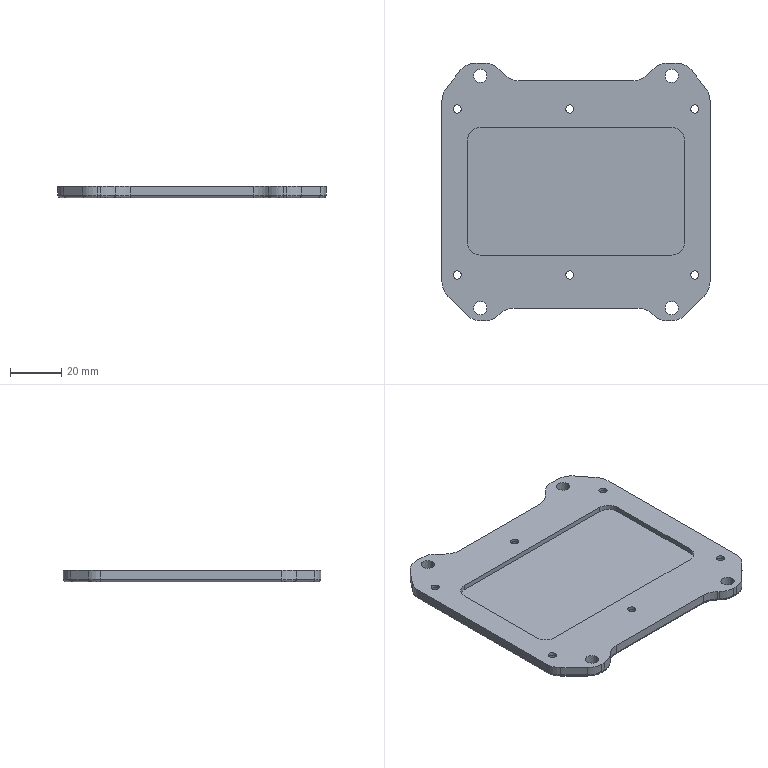NC program | NX | posted with a generic post | part box 105 x 101 x 4.5 mm
Lines 3985 to 4891 of 30641:
(CURVE_DRIVE , TOOL : 球刀R1-4-D4-50)
N7932 T08 M6
N7934 G53
N7936 G17 G0 G90 X36.658 Y51.5 S4500 M3
N7938 G43 Z20. H8
N7940 Z2.579
N7942 G94 G1 Z-1. F2500.
N7944 X36.668 Z-1.142
N7946 X36.698 Z-1.282
N7948 X36.748 Z-1.415
N7950 X36.817 Z-1.541
N7952 X36.902 Z-1.655
N7954 X37.003 Z-1.756
N7956 X37.117 Z-1.841
N7958 X37.242 Z-1.91
N7960 X37.376 Z-1.959
N7962 X37.516 Z-1.99
N7964 X37.658 Z-2.
N7966 X39.193
N7968 X39.348 Y51.498
N7970 X39.503 Y51.494
N7972 X39.658 Y51.488
N7974 X39.968 Y51.466
N7976 X40.157 Y51.447
N7978 X40.433 Y51.413
N7980 G2 X46.277 Y48.043 R9.005
N7982 G1 X51.587 Y41.282
N7984 G2 X53.5 Y35.665 R9.008
N7986 G1 Y-35.201
N7988 G2 X51.02 Y-41.39 R9.002
N7990 G1 X50.864 Y-41.55 Z-2.001
N7992 X50.843 Y-41.571 Z-2.007
N7994 X50.825 Y-41.589 Z-2.003
N7996 X43.531 Y-48.883 Z-2.
N7998 G2 X40.952 Y-50.674 R9.036
N8000 G1 X40.897 Y-50.699 Z-2.001
N8002 X40.833 Y-50.727 Z-2.002
N8004 X40.688 Y-50.79 Z-2.001
N8006 X40.588 Y-50.832 Z-2.
N8008 X40.433 Y-50.894
N8010 G2 X37.18 Y-51.5 R9.002
N8012 G1 X35.785
N8014 G2 X29.434 Y-48.848 R9.004
N8016 G1 X29.124 Y-48.539
N8018 G3 X24.39 Y-46.504 R6.999
N8020 G1 X24.322 Y-46.502 Z-2.001
N8022 X24.167 Y-46.5 Z-2.004
N8024 X24.08 Z-2.006
N8026 X23.925 Z-2.002
N8028 X-24.167 Z-2.
N8030 G3 X-29.124 Y-48.539 R7.002
N8032 G1 X-29.434 Y-48.848
N8034 G2 X-31.912 Y-50.61 R9.023
N8036 G1 X-32.048 Y-50.674 Z-2.001
N8038 X-32.167 Y-50.727 Z-2.002
N8040 X-32.222 Y-50.752 Z-2.001
N8042 X-32.377 Y-50.818 Z-2.
N8044 X-32.532 Y-50.88
N8046 G2 X-35.785 Y-51.5 R9.056
N8048 G1 X-37.18
N8050 G2 X-43.531 Y-48.883 R9.005
N8052 G1 X-50.87 Y-41.545
N8054 G2 X-53.5 Y-35.201 R9.006
N8056 G1 Y35.665
N8058 G2 X-51.502 Y41.39 R9.017
N8060 G1 X-46.277 Y48.043
N8062 G2 X-40.433 Y51.413 R9.005
N8064 G1 X-40.158 Y51.447
N8066 X-39.968 Y51.466
N8068 X-39.658 Y51.488
N8070 X-39.503 Y51.494
N8072 X-39.348 Y51.498
N8074 X-39.193 Y51.5
N8076 X-35.785
N8078 G2 X-29.434 Y48.848 R9.004
N8080 G1 X-27.236 Y46.651
N8082 G3 X-25.641 Y45.413 R7.073
N8084 G1 X-25.561 Y45.368
N8086 G3 X-22.153 Y44.5 R6.993
N8088 G1 X22.153
N8090 G3 X27.11 Y46.525 R6.998
N8092 G1 X27.786 Y47.2
N8094 X29.434 Y48.848
N8096 G2 X31.912 Y50.61 R9.023
N8098 G1 X32.048 Y50.674 Z-2.001
N8100 X32.167 Y50.727 Z-2.002
N8102 X32.222 Y50.752 Z-2.001
N8104 X32.287 Y50.78 Z-2.
N8106 G2 X35.785 Y51.5 R8.987
N8108 G1 X37.658
N8110 Y51.499 Z-1.969
N8112 Y51.497 Z-1.92
N8114 X39.193
N8116 X39.348 Y51.495
N8118 X39.503 Y51.491
N8120 X39.658 Y51.485
N8122 X39.968 Y51.463
N8124 X40.154 Y51.445
N8126 X40.356 Y51.42
N8128 G2 X42.137 Y51. R9.113
N8130 G1 X42.187 Y50.983
N8132 G2 X43.267 Y50.519 R9.54
N8134 G1 X43.376 Y50.462
N8136 X43.55 Y50.368
N8138 X43.558 Y50.364
N8140 G2 X44.303 Y49.9 R8.898
N8142 G1 X44.461 Y49.789
N8144 G2 X46.303 Y48.006 R9.094
N8146 G1 X46.638 Y47.579
N8148 G3 X48.825 Y44.794 R3917.638
N8150 G1 X48.947 Y44.639
N8152 X48.953 Y44.631
N8154 X49.56 Y43.859
N8156 X49.676 Y43.711
N8158 G2 X50.988 Y42.04 R9051.305
N8160 G1 X51.255 Y41.699
N8162 G2 X51.742 Y41.074 R21.302
N8164 G1 X51.794 Y40.999
N8166 G2 X52.655 Y39.533 R8.658
N8168 G1 X52.667 Y39.511
N8170 G2 X53.291 Y37.654 R9.165
N8172 G1 X53.3 Y37.601
N8174 G2 X53.493 Y35.974 R8.95
N8176 G1 X53.495 Y35.896
N8178 X53.497 Y35.82
N8180 X53.496 Y35.746
N8182 X53.497 Y35.665
N8184 Y-35.201
N8186 G2 X53.462 Y-35.974 R8.462
N8188 G1 X53.445 Y-36.159
N8190 G2 X53.051 Y-37.986 R8.987
N8192 G1 X52.989 Y-38.166
N8194 X52.981 Y-38.192
N8196 G2 X51.288 Y-41.092 R9.015
N8198 G1 X51.161 Y-41.235
N8200 X51.017 Y-41.39
N8202 X50.866 Y-41.545 Z-1.921
N8204 X50.836 Y-41.575 Z-1.925
N8206 X50.812 Y-41.599 Z-1.923
N8208 X43.593 Y-48.817 Z-1.92
N8210 G2 X41.003 Y-50.646 R9.001
N8212 G1 X40.932 Y-50.681
N8214 X40.814 Y-50.733 Z-1.922
N8216 X40.715 Y-50.776 Z-1.921
N8218 X40.687 Y-50.787
N8220 X40.592 Y-50.829 Z-1.92
N8222 X40.588 Y-50.83
N8224 X40.433 Y-50.891
N8226 G2 X38.884 Y-51.336 R8.857
N8228 G1 X38.794 Y-51.352
N8230 G2 X37.18 Y-51.497 R8.944
N8232 G1 X35.785
N8234 G2 X33.839 Y-51.278 R8.977
N8236 G1 X33.678 Y-51.239
N8238 G2 X31.448 Y-50.366 R8.951
N8240 G1 X31.442 Y-50.364
N8242 X31.381 Y-50.328
N8244 G2 X30.318 Y-49.624 R8.845
N8246 G1 X30.249 Y-49.57
N8248 G2 X29.872 Y-49.256 R8.905
N8250 G1 X29.826 Y-49.214
N8252 X29.744 Y-49.14
N8254 X29.735 Y-49.133
N8256 X29.578 Y-48.985
N8258 X29.406 Y-48.817
N8260 X29.124 Y-48.535
N8262 G3 X25.096 Y-46.557 R7.005
N8264 G1 X24.941 Y-46.538
N8266 X24.786 Y-46.524
N8268 X24.631 Y-46.512
N8270 X24.477 Y-46.504
N8272 X24.393 Y-46.501
N8274 X24.322 Y-46.499 Z-1.921
N8276 X24.243 Z-1.922
N8278 X24.167 Y-46.498 Z-1.924
N8280 X24.085 Z-1.926
N8282 X23.925 Z-1.922
N8284 X-24.167 Z-1.92
N8286 G3 X-26.955 Y-47.068 R7.018
N8288 G1 X-27.077 Y-47.123
N8290 X-27.11 Y-47.137
N8292 G3 X-29.124 Y-48.535 R7.012
N8294 G1 X-29.434 Y-48.844
N8296 G2 X-30.082 Y-49.436 R10.496
N8298 G1 X-30.147 Y-49.487
N8300 G2 X-30.495 Y-49.756 R6.75
N8302 G1 X-30.518 Y-49.773
N8304 G2 X-31.381 Y-50.328 R8.373
N8306 G1 X-31.445 Y-50.365
N8308 X-31.448 Y-50.366
N8310 X-31.603 Y-50.451
N8312 X-31.733 Y-50.519
N8314 X-31.741 Y-50.522
N8316 X-31.912 Y-50.607
N8318 X-32.062 Y-50.678 Z-1.921
N8320 X-32.067 Y-50.679
N8322 X-32.146 Y-50.715 Z-1.922
N8324 X-32.222 Y-50.749
N8326 X-32.276 Y-50.771 Z-1.921
N8328 X-32.377 Y-50.815
N8330 X-32.409 Y-50.828 Z-1.92
N8332 X-32.532 Y-50.877
N8334 G2 X-34.856 Y-51.446 R8.986
N8336 G1 X-34.863 Y-51.447
N8338 G2 X-35.785 Y-51.497 R9.145
N8340 G1 X-37.18
N8342 G2 X-40.588 Y-50.83 R8.992
N8344 G1 X-40.595 Y-50.827
N8346 G2 X-41.052 Y-50.624 R13.008
N8348 G1 X-41.245 Y-50.529
N8350 X-41.267 Y-50.519
N8352 G2 X-42.295 Y-49.906 R9.146
N8354 G1 X-42.495 Y-49.765
N8356 G2 X-43.531 Y-48.879 R9.388
N8358 G1 X-46.378 Y-46.032
N8360 X-50.866 Y-41.545
N8362 G2 X-53.229 Y-37.367 R9.014
N8364 G1 X-53.245 Y-37.296
N8366 G2 X-53.474 Y-35.82 R8.914
N8368 G1 X-53.484 Y-35.665
N8370 X-53.49 Y-35.51
N8372 X-53.495 Y-35.356
N8374 X-53.497 Y-35.201
N8376 Y35.665
N8378 G2 X-53.445 Y36.706 R9.699
N8380 G1 X-53.433 Y36.802
N8382 G2 X-53.196 Y38.039 R8.303
N8384 G1 X-53.17 Y38.141
N8386 G2 X-52.856 Y39.069 R9.602
N8388 G1 X-52.82 Y39.159
N8390 G2 X-51.896 Y40.857 R9.054
N8392 G1 X-51.848 Y40.926
N8394 G2 X-51.267 Y41.684 R16.261
N8396 G1 X-51.126 Y41.864
N8398 G2 X-49.708 Y43.67 R1437.629
N8400 G1 X-49.573 Y43.842
N8402 G3 X-47.249 Y46.802 R3035.735
N8404 G1 X-47.124 Y46.96
N8406 X-47.094 Y46.999
N8408 X-46.759 Y47.424
N8410 X-46.635 Y47.583
N8412 X-46.303 Y48.006
N8414 G2 X-45.39 Y49.016 R9.198
N8416 G1 X-45.332 Y49.07
N8418 G2 X-43.686 Y50.291 R8.897
N8420 G1 X-43.558 Y50.364
N8422 X-43.55 Y50.368
N8424 G2 X-42.941 Y50.677 R8.914
N8426 G1 X-42.86 Y50.712
N8428 G2 X-41.982 Y51.052 R9.144
N8430 G1 X-41.914 Y51.072
N8432 X-41.706 Y51.138
N8434 G2 X-40.278 Y51.43 R9.209
N8436 G1 X-40.138 Y51.447
N8438 X-39.968 Y51.463
N8440 X-39.658 Y51.485
N8442 X-39.503 Y51.491
N8444 X-39.348 Y51.495
N8446 X-39.193 Y51.497
N8448 X-35.785
N8450 G2 X-33.839 Y51.278 R8.977
N8452 G1 X-33.678 Y51.239
N8454 G2 X-31.448 Y50.366 R8.951
N8456 G1 X-31.442 Y50.364
N8458 X-31.381 Y50.328
N8460 G2 X-30.318 Y49.624 R8.845
N8462 G1 X-30.249 Y49.57
N8464 G2 X-29.872 Y49.256 R8.905
N8466 G1 X-29.826 Y49.214
N8468 X-29.744 Y49.14
N8470 X-29.735 Y49.133
N8472 X-29.578 Y48.985
N8474 X-29.406 Y48.817
N8476 X-27.24 Y46.651
N8478 G3 X-25.871 Y45.546 R7.094
N8480 G1 X-25.8 Y45.504
N8482 G3 X-23.492 Y44.621 R6.981
N8484 G1 X-23.392 Y44.602
N8486 G3 X-22.153 Y44.498 R7.183
N8488 G1 X22.153
N8490 G3 X24.199 Y44.794 R6.901
N8492 G1 X24.322 Y44.831
N8494 G3 X27.099 Y46.51 R7.007
N8496 G1 X27.33 Y46.741
N8498 X29.434 Y48.844
N8500 G2 X30.082 Y49.436 R10.496
N8502 G1 X30.147 Y49.487
N8504 G2 X30.495 Y49.756 R6.751
N8506 G1 X30.518 Y49.773
N8508 G2 X31.381 Y50.328 R8.374
N8510 G1 X31.445 Y50.365
N8512 X31.448 Y50.366
N8514 X31.603 Y50.451
N8516 X31.733 Y50.519
N8518 X31.741 Y50.522
N8520 X31.912 Y50.607
N8522 X32.062 Y50.678 Z-1.921
N8524 X32.067 Y50.679
N8526 X32.146 Y50.715 Z-1.922
N8528 X32.222 Y50.749 Z-1.921
N8530 X32.277 Y50.772 Z-1.92
N8532 X32.377 Y50.815
N8534 X32.409 Y50.828
N8536 X32.532 Y50.877
N8538 G2 X34.856 Y51.446 R8.986
N8540 G1 X34.863 Y51.447
N8542 G2 X35.785 Y51.497 R9.145
N8544 G1 X37.658
N8546 Y51.493 Z-1.84
N8548 X39.191
N8550 X39.348 Y51.491
N8552 X39.537 Y51.486
N8554 X39.658 Y51.481
N8556 X39.871 Y51.466
N8558 X39.968 Y51.459
N8560 X40.087 Y51.447
N8562 X40.278 Y51.426
N8564 X40.433 Y51.406
N8566 G2 X42.791 Y50.737 R8.941
N8568 G1 X42.925 Y50.679
N8570 G2 X46.292 Y48.013 R9.018
N8572 G1 X47.483 Y46.496
N8574 X49.966 Y43.334
N8576 X50.037 Y43.243
N8578 X50.396 Y42.787
N8580 X51.587 Y41.271
N8582 G2 X53.129 Y38.265 R8.995
N8584 G1 X53.153 Y38.183
N8586 G2 X53.493 Y35.665 R8.998
N8588 G1 Y-35.201
N8590 G2 X51.011 Y-41.39 R9.
N8592 G1 X50.86 Y-41.545 Z-1.841
N8594 X50.849 Y-41.556 Z-1.843
N8596 X50.784 Y-41.621
N8598 X43.519 Y-48.886 Z-1.84
N8600 G2 X41.052 Y-50.62 R9.021
N8602 G1 X40.898 Y-50.691 Z-1.841
N8604 X40.743 Y-50.76
N8606 X40.656 Y-50.796
N8608 X40.619 Y-50.811
N8610 X40.578 Y-50.828 Z-1.84
N8612 X40.433 Y-50.887
N8614 G2 X37.182 Y-51.493 R9.021
N8616 G1 X35.788
N8618 G2 X29.415 Y-48.82 R9.001
N8620 G1 X29.104 Y-48.51
N8622 G3 X24.477 Y-46.5 R7.006
N8624 G1 X24.322 Y-46.495 Z-1.841
N8626 X24.167 Y-46.493 Z-1.844
N8628 X24.124 Z-1.845
N8630 X24.012 Z-1.844
N8632 X23.966 Z-1.843
N8634 X23.857 Z-1.842
N8636 X-24.167 Z-1.84
N8638 G3 X-29.124 Y-48.529 R7.014
N8640 G1 X-29.434 Y-48.839
N8642 G2 X-31.912 Y-50.602 R8.989
N8644 G1 X-32.064 Y-50.674 Z-1.841
N8646 X-32.067 Y-50.675
N8648 X-32.139 Y-50.707 Z-1.842
N8650 X-32.222 Y-50.745
N8652 X-32.298 Y-50.777 Z-1.841
N8654 X-32.377 Y-50.81
N8656 X-32.41 Y-50.824 Z-1.84
N8658 X-32.532 Y-50.873
N8660 G2 X-35.785 Y-51.493 R9.042
N8662 G1 X-37.18
N8664 G2 X-43.531 Y-48.874 R9.002
N8666 G1 X-50.86 Y-41.545
N8668 G2 X-53.493 Y-35.201 R8.997
N8670 G1 Y35.683
N8672 G2 X-51.587 Y41.271 R9.003
N8674 G1 X-50.159 Y43.089
N8676 X-50.035 Y43.247
N8678 X-49.227 Y44.276
N8680 X-47.404 Y46.597
N8682 X-46.268 Y48.043
N8684 G2 X-42.925 Y50.679 R9.013
N8686 G1 X-42.791 Y50.737
N8688 X-42.756 Y50.753
N8690 G2 X-40.278 Y51.426 R8.982
N8692 G1 X-40.068 Y51.449
N8694 X-39.968 Y51.459
N8696 X-39.752 Y51.475
N8698 X-39.658 Y51.481
N8700 X-39.481 Y51.488
N8702 X-39.348 Y51.491
N8704 X-39.193 Y51.493
N8706 X-35.788
N8708 G2 X-29.415 Y48.82 R9.001
N8710 G1 X-27.153 Y46.559
N8712 G3 X-22.153 Y44.493 R7.009
N8714 G1 X22.153
N8716 G3 X27.11 Y46.516 R7.013
N8718 G1 X27.415 Y46.82
N8720 X29.434 Y48.839
N8722 G2 X31.912 Y50.602 R8.989
N8724 G1 X32.064 Y50.674 Z-1.841
N8726 X32.067 Y50.675
N8728 X32.139 Y50.707 Z-1.842
N8730 X32.222 Y50.745 Z-1.841
N8732 X32.301 Y50.778 Z-1.84
N8734 G2 X35.785 Y51.493 R8.987
N8736 G1 X37.658
N8738 Y51.486 Z-1.766
N8740 Y51.485 Z-1.761
N8742 X39.193
N8744 X39.348 Y51.483
N8746 X39.503 Y51.479
N8748 X39.658 Y51.472
N8750 X39.712 Y51.468
N8752 X39.821 Y51.462 Z-1.76
N8754 G2 X40.445 Y51.396 R9.361
N8756 G1 X40.588 Y51.374 Z-1.761
N8758 G2 X46.137 Y48.193 R8.982
N8760 G1 X46.311 Y47.975
N8762 G3 X47.503 Y46.457 R4301.774
N8764 G1 X47.959 Y45.877
N8766 G3 X49.903 Y43.401 R4715.511
N8768 G1 X50.024 Y43.247
N8770 G2 X51.604 Y41.235 R6903.767
N8772 G1 X51.724 Y41.076
N8774 X51.832 Y40.926
N8776 X51.896 Y40.835
N8778 X51.94 Y40.771
N8780 X51.991 Y40.691
N8782 G2 X52.361 Y40.085 R7.942
N8784 G1 X52.408 Y39.998
N8786 G2 X53.485 Y35.665 R8.992
N8788 G1 Y-35.201
N8790 G2 X52.527 Y-39.224 R8.99
N8792 G1 X52.446 Y-39.378
N8794 G2 X51.144 Y-41.235 R9.011
N8796 G1 X50.984 Y-41.406
N8798 X50.848 Y-41.545 Z-1.762
N8800 X50.812 Y-41.581 Z-1.764
N8802 X43.576 Y-48.817 Z-1.761
N8804 G2 X41.052 Y-50.61 R9.018
N8806 G1 X40.898 Y-50.682
N8808 X40.743 Y-50.751 Z-1.762
N8810 X40.655 Y-50.788 Z-1.761
N8812 X40.556 Y-50.828
N8814 X40.433 Y-50.878
N8816 G2 X37.18 Y-51.485 R9.009
N8818 G1 X35.785
N8820 G2 X33.94 Y-51.286 R8.991
N8822 G1 X33.926 Y-51.282
N8824 X33.841 Y-51.266
N8826 G2 X30.286 Y-49.583 R9.008
N8828 G1 X30.102 Y-49.436
N8830 G2 X29.434 Y-48.826 R8.969
N8832 G1 X29.124 Y-48.517
N8834 G3 X24.477 Y-46.491 R7.019
N8836 G1 X24.322 Y-46.487 Z-1.762
N8838 X24.154 Y-46.485 Z-1.765
N8840 X23.998
N8842 X23.857 Z-1.763
N8844 X-24.167 Z-1.761
N8846 G3 X-29.124 Y-48.517 R7.019
N8848 G1 X-29.434 Y-48.826
N8850 G2 X-31.912 Y-50.593 R8.963
N8852 G1 X-32.067 Y-50.665 Z-1.762
N8854 X-32.084 Y-50.674
N8856 X-32.222 Y-50.735
N8858 X-32.404 Y-50.813 Z-1.761
N8860 X-32.532 Y-50.864
N8862 G2 X-33.841 Y-51.266 R9.054
N8864 G1 X-33.926 Y-51.282
N8866 X-33.94 Y-51.286
N8868 G2 X-35.785 Y-51.485 R8.931
N8870 G1 X-37.204 Y-51.484
N8872 G2 X-43.531 Y-48.862 R8.986
N8874 G1 X-50.848 Y-41.545
N8876 G2 X-52.985 Y-38.141 R8.968
N8878 G1 X-53.037 Y-37.986
N8880 G2 X-53.485 Y-35.201 R9.018
N8882 G1 Y35.665
N8884 G2 X-52.968 Y38.737 R8.983
N8886 G1 X-52.903 Y38.914
N8888 G2 X-51.991 Y40.691 R8.774
N8890 G1 X-51.94 Y40.771
N8892 X-51.885 Y40.852
N8894 X-51.832 Y40.926
N8896 X-51.721 Y41.08
N8898 X-51.587 Y41.257
N8900 G2 X-50.037 Y43.23 R3006.597
N8902 G1 X-50.024 Y43.247
N8904 G2 X-48.643 Y45.005 R1093.849
N8906 G1 X-48.333 Y45.4
N8908 X-48.323 Y45.413
N8910 G3 X-46.501 Y47.734 R7264.617
N8912 G1 X-46.257 Y48.043
N8914 G2 X-40.278 Y51.418 R8.983
N8916 G1 X-40.204 Y51.426 Z-1.76
N8918 X-40.123 Y51.435
N8920 X-39.968 Y51.45
N8922 X-39.813 Y51.462
N8924 X-39.712 Y51.468 Z-1.761
N8926 X-39.658 Y51.472
N8928 X-39.503 Y51.479
N8930 X-39.348 Y51.483
N8932 X-39.193 Y51.485
N8934 X-35.785
N8936 G2 X-33.94 Y51.286 R8.991
N8938 G1 X-33.926 Y51.282
N8940 X-33.841 Y51.266
N8942 G2 X-30.286 Y49.583 R9.008
N8944 G1 X-30.102 Y49.436
N8946 G2 X-29.434 Y48.826 R8.969
N8948 G1 X-27.182 Y46.575
N8950 G3 X-22.153 Y44.485 R7.018
N8952 G1 X22.169
N8954 G3 X27.11 Y46.504 R7.015
N8956 G1 X27.258 Y46.651
N8958 X29.434 Y48.826
N8960 G2 X31.912 Y50.593 R8.963
N8962 G1 X32.067 Y50.665 Z-1.762
N8964 X32.084 Y50.674
N8966 X32.178 Y50.715
N8968 X32.222 Y50.735
N8970 X32.377 Y50.802 Z-1.761
N8972 G2 X33.841 Y51.266 R9.075
N8974 G1 X33.926 Y51.282
N8976 X33.94 Y51.286
N8978 G2 X35.785 Y51.485 R8.931
N8980 G1 X37.658
N8982 Y51.474 Z-1.681
N8984 X39.192
N8986 X39.348 Y51.472
N8988 X39.537 Y51.465
N8990 X39.693 Y51.458
N8992 X39.859 Y51.447
N8994 X39.968 Y51.439
N8996 X40.123 Y51.423
N8998 X40.216 Y51.412
N9000 G2 X41.859 Y51.065 R8.766
N9002 G1 X41.919 Y51.045 Z-1.682
N9004 X41.982 Y51.026 Z-1.681
N9006 G2 X46.243 Y48.043 R8.989
N9008 G1 X46.279 Y47.998
N9010 G2 X47.249 Y46.763 R2907.259
N9012 G1 X47.351 Y46.634
N9014 G3 X49.058 Y44.46 R1068.571
N9016 G1 X49.159 Y44.33
N9018 G2 X51.589 Y41.235 R6511.103
N9020 G1 X51.723 Y41.058
N9022 G2 X52.89 Y38.914 R8.918
N9024 G1 X52.924 Y38.819 Z-1.682
N9026 X52.947 Y38.76 Z-1.681
N9028 G2 X53.474 Y35.665 R8.988
N9030 G1 Y-35.213
N9032 X53.472 Y-35.356
N9034 G2 X53.438 Y-35.974 R9.551
N9036 G1 X53.432 Y-36.029 Z-1.682
N9038 X53.421 Y-36.148 Z-1.681
N9040 G2 X51.043 Y-41.325 R8.968
N9042 G1 X50.967 Y-41.406 Z-1.682
N9044 X50.911 Y-41.463
N9046 X50.833 Y-41.545 Z-1.683
N9048 X50.812 Y-41.566 Z-1.684
N9050 X43.531 Y-48.846 Z-1.681
N9052 X43.432 Y-48.941 Z-1.682
N9054 X43.401 Y-48.972 Z-1.681
N9056 G2 X41.052 Y-50.597 R8.979
N9058 G1 X40.888 Y-50.674 Z-1.682
N9060 X40.743 Y-50.738 Z-1.683
N9062 X40.679 Y-50.766 Z-1.682
N9064 X40.551 Y-50.818
N9066 X40.433 Y-50.865 Z-1.681
N9068 G2 X37.334 Y-51.472 R9.002
N9070 G1 X37.181 Y-51.474
N9072 X35.785
N9074 X35.63 Y-51.471
N9076 X35.475 Y-51.466
N9078 G2 X33.462 Y-51.159 R8.897
N9080 G1 X33.384 Y-51.138
N9082 X33.145 Y-51.067
N9084 X33.069 Y-51.042 Z-1.682
N9086 X32.997 Y-51.02 Z-1.681
N9088 G2 X31.448 Y-50.339 R8.978
N9090 G1 X31.411 Y-50.317 Z-1.682
N9092 G2 X30.828 Y-49.96 R7.452
N9094 G1 X30.673 Y-49.855 Z-1.681
N9096 G2 X29.439 Y-48.817 R9.193
N9098 G1 X29.124 Y-48.502
N9100 X28.962 Y-48.346
N9102 G3 X24.477 Y-46.48 R7.026
N9104 G1 X24.322 Y-46.475 Z-1.682
N9106 X24.152 Z-1.685
N9108 X23.997
N9110 X23.857 Y-46.474 Z-1.684
N9112 X-24.167 Z-1.681
N9114 X-24.331 Y-46.475
N9116 G3 X-29.129 Y-48.507 R7.022
N9118 G1 X-29.439 Y-48.817
N9120 X-29.598 Y-48.972
N9122 X-29.639 Y-49.009
N9124 G2 X-31.603 Y-50.423 R8.933
N9126 G1 X-31.758 Y-50.504
N9128 X-31.845 Y-50.547
N9130 X-32.077 Y-50.658 Z-1.682
N9132 X-32.151 Y-50.692 Z-1.683
N9134 X-32.222 Y-50.723
N9136 X-32.377 Y-50.789 Z-1.682
N9138 X-32.532 Y-50.851 Z-1.681
N9140 G2 X-35.321 Y-51.459 R9.021
N9142 G1 X-35.37 Y-51.461 Z-1.682
N9144 X-35.515 Y-51.467 Z-1.681
N9146 X-35.63 Y-51.471
N9148 X-35.785 Y-51.474
N9150 X-37.18
N9152 X-37.34 Y-51.472
N9154 X-37.489 Y-51.467
N9156 X-37.603 Y-51.462 Z-1.682
N9158 X-37.644 Y-51.461 Z-1.681
N9160 X-37.831 Y-51.45
N9162 G2 X-40.709 Y-50.752 R8.984
N9164 G1 X-40.898 Y-50.669
N9166 G2 X-43.432 Y-48.941 R8.984
N9168 G1 X-43.531 Y-48.846
N9170 X-50.832 Y-41.545
N9172 X-50.91 Y-41.464 Z-1.682
N9174 G2 X-53.257 Y-37.142 R8.971
N9176 G1 X-53.29 Y-36.987 Z-1.681
N9178 G2 X-53.423 Y-36.129 R9.035
N9180 G1 X-53.432 Y-36.029 Z-1.682
N9182 X-53.438 Y-35.974 Z-1.681
N9184 G2 X-53.474 Y-35.201 R9.524
N9186 G1 Y35.665
N9188 G2 X-53.27 Y37.632 R9.043
N9190 G1 X-53.246 Y37.734
N9192 G2 X-52.767 Y39.224 R9.021
N9194 G1 X-52.7 Y39.378
N9196 G2 X-51.589 Y41.235 R9.052
N9198 G1 X-51.413 Y41.462
N9200 G2 X-50.497 Y42.628 R2231.241
N9202 G1 X-50.332 Y42.837
N9204 G3 X-48.432 Y45.258 R9957.25
N9206 G1 X-48.309 Y45.413
N9208 G2 X-46.32 Y47.946 R8088.524
N9210 G1 X-46.279 Y47.998
N9212 G2 X-45.39 Y48.983 R9.571
N9214 G1 X-45.327 Y49.041 Z-1.682
N9216 X-45.235 Y49.128 Z-1.681
N9218 G2 X-42.269 Y50.926 R8.979
N9220 G1 X-42.198 Y50.951 Z-1.682
N9222 X-42.11 Y50.983 Z-1.681
N9224 X-41.982 Y51.026
N9226 G2 X-40.216 Y51.412 R8.767
N9228 G1 X-40.123 Y51.423
N9230 X-39.968 Y51.439
N9232 X-39.813 Y51.451
N9234 X-39.693 Y51.458
N9236 X-39.503 Y51.467 Z-1.682
N9238 X-39.348 Y51.472 Z-1.681
N9240 X-39.193 Y51.474
N9242 X-35.785
N9244 X-35.63 Y51.471
N9246 X-35.475 Y51.466
N9248 G2 X-33.462 Y51.159 R8.897
N9250 G1 X-33.384 Y51.138
N9252 X-33.145 Y51.067
N9254 X-33.069 Y51.042 Z-1.682
N9256 X-32.997 Y51.02 Z-1.681
N9258 G2 X-31.448 Y50.339 R8.978
N9260 G1 X-31.411 Y50.317 Z-1.682
N9262 G2 X-30.828 Y49.96 R7.452
N9264 G1 X-30.673 Y49.855 Z-1.681
N9266 G2 X-29.439 Y48.817 R9.193
N9268 G1 X-27.175 Y46.552
N9270 X-27.11 Y46.488
N9272 G3 X-26.49 Y45.946 R7.059
N9274 G1 X-26.4 Y45.877 Z-1.682
N9276 G3 X-22.153 Y44.473 R7.038
N9278 G1 X22.153 Z-1.681
N9280 G3 X27.118 Y46.496 R7.025
N9282 G1 X27.537 Y46.914
N9284 X29.439 Y48.817
N9286 X29.598 Y48.972
N9288 X29.639 Y49.009
N9290 G2 X31.603 Y50.423 R8.933
N9292 G1 X31.758 Y50.504
N9294 X31.845 Y50.547
N9296 X32.077 Y50.658 Z-1.682
N9298 X32.151 Y50.691 Z-1.683
N9300 X32.222 Y50.723 Z-1.682
N9302 X32.377 Y50.789 Z-1.681
N9304 G2 X35.321 Y51.459 R9.031
N9306 G1 X35.37 Y51.461 Z-1.682
N9308 X35.515 Y51.467 Z-1.681
N9310 X35.63 Y51.471
N9312 X35.785 Y51.474
N9314 X37.658
N9316 Y51.458 Z-1.603
N9318 X39.193
N9320 X39.363
N9322 X39.658 Y51.447 Z-1.602
N9324 X39.764 Y51.44
N9326 X39.881 Y51.43 Z-1.603
N9328 X39.968 Y51.425 Z-1.602
N9330 X40.123 Y51.41
N9332 X40.163 Y51.406
N9334 X40.356 Y51.382
N9336 X40.433 Y51.372 Z-1.603
N9338 G2 X41.879 Y51.045 R8.825
N9340 G1 X41.982 Y51.011
N9342 X42.036 Y50.994
N9344 G2 X43.421 Y50.395 R9.042
N9346 G1 X43.491 Y50.356
N9348 X43.531 Y50.335
N9350 X43.638 Y50.275
N9352 X43.78 Y50.192
N9354 X43.841 Y50.155
N9356 X43.878 Y50.131
N9358 X44.003 Y50.055
N9360 X44.189 Y49.932
N9362 X44.259 Y49.885
N9364 X44.306 Y49.851
N9366 X44.456 Y49.745
N9368 X44.615 Y49.627
N9370 G2 X46.248 Y48.014 R8.979
N9372 G1 X46.334 Y47.904
N9374 X46.345 Y47.889
N9376 X46.59 Y47.579
N9378 X46.629 Y47.528
N9380 X46.71 Y47.427
N9382 X47.119 Y46.905
N9384 X47.316 Y46.653
N9386 X47.362 Y46.595
N9388 G3 X48.333 Y45.359 R1077.718
N9390 G1 X48.411 Y45.258
N9392 X48.488 Y45.162
N9394 X48.643 Y44.965
N9396 X48.654 Y44.949
N9398 X48.781 Y44.79
N9400 X48.798 Y44.766
N9402 X48.905 Y44.631
N9404 G3 X49.778 Y43.519 R291.457
N9406 G1 X49.869 Y43.401
N9408 X49.883 Y43.387
N9410 X49.992 Y43.247
N9412 X50.041 Y43.185
N9414 X50.113 Y43.092
N9416 X50.171 Y43.019
N9418 X50.269 Y42.895
N9420 X50.356 Y42.782
N9422 X50.49 Y42.613
N9424 X50.502 Y42.597
N9426 X50.655 Y42.403
N9428 G2 X51.451 Y41.39 R406.68
N9430 G1 X51.587 Y41.216
N9432 G2 X52.981 Y38.623 R9.051
N9434 G1 X52.986 Y38.605
N9436 X53.015 Y38.519
N9438 G2 X53.263 Y37.598 R8.544
N9440 G1 X53.27 Y37.561
N9442 X53.285 Y37.495
N9444 G2 X53.41 Y36.672 R8.959
N9446 G1 X53.414 Y36.621
N9448 X53.417 Y36.593
N9450 X53.422 Y36.534
N9452 X53.434 Y36.41
N9454 X53.437 Y36.362
N9456 X53.442 Y36.299
N9458 X53.446 Y36.234
N9460 X53.456 Y35.974
N9462 X53.458 Y35.665
N9464 Y-35.201
N9466 Y-35.356
N9468 X53.452 Y-35.546
N9470 X53.446 Y-35.685
N9472 X53.436 Y-35.82
N9474 X53.431 Y-35.877
N9476 X53.424 Y-35.981
N9478 G2 X53.291 Y-36.919 R9.991
N9480 G1 X53.261 Y-37.058
N9482 X53.243 Y-37.144
N9484 X53.226 Y-37.212
N9486 X53.215 Y-37.262
N9488 G2 X52.598 Y-39.019 R8.982
N9490 G1 X52.573 Y-39.069
N9492 X52.516 Y-39.189
N9494 G2 X52.154 Y-39.843 R9.595
N9496 G1 X52.127 Y-39.885
N9498 X52.057 Y-39.997
N9500 X52.051 Y-40.008
N9502 G2 X50.967 Y-41.387 R9.068
N9504 G1 X50.819 Y-41.539 Z-1.605
N9506 X50.805 Y-41.553
N9508 X43.531 Y-48.825 Z-1.603
N9510 X43.503 Y-48.852
N9512 X43.382 Y-48.972
N9514 X43.376 Y-48.978
N9516 G2 X42.456 Y-49.745 R8.854
N9518 G1 X42.447 Y-49.751
N9520 X42.288 Y-49.865 Z-1.602
N9522 G2 X41.362 Y-50.427 R8.867
N9524 G1 X41.305 Y-50.455 Z-1.603
N9526 X41.183 Y-50.519
N9528 X41.052 Y-50.582
N9530 X40.856 Y-50.674
N9532 X40.726 Y-50.731 Z-1.604
N9534 X40.58 Y-50.792 Z-1.603
N9536 X40.433 Y-50.85
N9538 G2 X39.733 Y-51.088 R7.909
N9540 G1 X39.566 Y-51.138 Z-1.602
N9542 X39.348 Y-51.195 Z-1.603
N9544 X39.193 Y-51.231
N9546 X39.078 Y-51.256
N9548 X39.039 Y-51.265
N9550 X38.909 Y-51.293 Z-1.602
N9552 X38.884 Y-51.296 Z-1.603
N9554 G2 X37.954 Y-51.426 R8.949
N9556 G1 X37.858 Y-51.433
N9558 X37.799 Y-51.438
N9560 X37.644 Y-51.448
N9562 X37.522 Y-51.452
N9564 X37.334 Y-51.458
N9566 X37.274
N9568 X37.18
N9570 X35.785
N9572 X35.63
N9574 X35.475 Y-51.452
N9576 X35.449 Y-51.451
N9578 X35.39 Y-51.449
N9580 X35.321 Y-51.446
N9582 X35.166 Y-51.435
N9584 X35.09 Y-51.428
N9586 X35.011 Y-51.423
N9588 X34.971 Y-51.418
N9590 X34.93 Y-51.415
N9592 G2 X33.825 Y-51.236 R8.976
N9594 G1 X33.738 Y-51.214
N9596 X33.617 Y-51.186
N9598 X33.551 Y-51.169
N9600 G2 X32.842 Y-50.951 R8.36
N9602 G1 X32.797 Y-50.935
N9604 X32.687 Y-50.896
N9606 X32.511 Y-50.828
N9608 X32.377 Y-50.773
N9610 X32.153 Y-50.678 Z-1.602
N9612 X32.144 Y-50.674
N9614 X32.124 Y-50.663 Z-1.603
N9616 X32.069 Y-50.639
N9618 G2 X31.419 Y-50.307 R9.144
N9620 G1 X31.325 Y-50.252
N9622 X31.293 Y-50.234
N9624 X31.25 Y-50.209
N9626 X31.138 Y-50.142
N9628 G2 X29.46 Y-48.817 R8.972
N9630 G1 X29.136 Y-48.494
N9632 G3 X27.65 Y-47.372 R6.97
N9634 G1 X27.575 Y-47.329
N9636 X27.487 Y-47.283
N9638 G3 X26.751 Y-46.945 R6.409
N9640 G1 X26.645 Y-46.903
N9642 X26.388 Y-46.813
N9644 G3 X26.026 Y-46.704 R9.808
N9646 G1 X25.863 Y-46.663
N9648 X25.716 Y-46.628
N9650 X25.561 Y-46.594
N9652 X25.398 Y-46.565
N9654 G3 X24.477 Y-46.465 R6.944
N9656 G1 X24.426 Y-46.464
N9658 X24.323 Y-46.461 Z-1.604
N9660 X24.167 Y-46.46 Z-1.606
N9662 X24.012 Z-1.607
N9664 X23.857 Z-1.605
N9666 X-24.167 Z-1.603
N9668 X-24.322 Y-46.461
N9670 G3 X-26.026 Y-46.704 R7.169
N9672 G1 X-26.098 Y-46.725
N9674 X-26.181 Y-46.748
N9676 X-26.247 Y-46.769
N9678 X-26.336 Y-46.796
N9680 X-26.388 Y-46.813
N9682 X-26.645 Y-46.903
N9684 X-26.751 Y-46.945
N9686 X-26.8 Y-46.963
N9688 G3 X-27.73 Y-47.416 R7.619
N9690 G1 X-27.845 Y-47.487
N9692 G3 X-29.15 Y-48.507 R6.982
N9694 G1 X-29.46 Y-48.817
N9696 X-29.618 Y-48.972
N9698 G2 X-30.142 Y-49.436 R10.416
N9700 G1 X-30.216 Y-49.495
N9702 G2 X-31.269 Y-50.221 R8.865
N9704 G1 X-31.293 Y-50.234
N9706 X-31.325 Y-50.252
N9708 X-31.419 Y-50.307
N9710 X-31.521 Y-50.364 Z-1.602
N9712 X-31.603 Y-50.409
N9714 X-31.774 Y-50.496 Z-1.603
N9716 X-31.921 Y-50.57
N9718 X-32.08 Y-50.644
N9720 X-32.124 Y-50.664 Z-1.604
N9722 X-32.143 Y-50.674
N9724 X-32.222 Y-50.708
N9726 X-32.377 Y-50.774 Z-1.603
N9728 X-32.532 Y-50.837
N9730 G2 X-33.738 Y-51.214 R8.721
N9732 G1 X-33.825 Y-51.236
N9734 X-33.876 Y-51.248
N9736 X-33.926 Y-51.258
N9738 G2 X-34.93 Y-51.415 R8.765